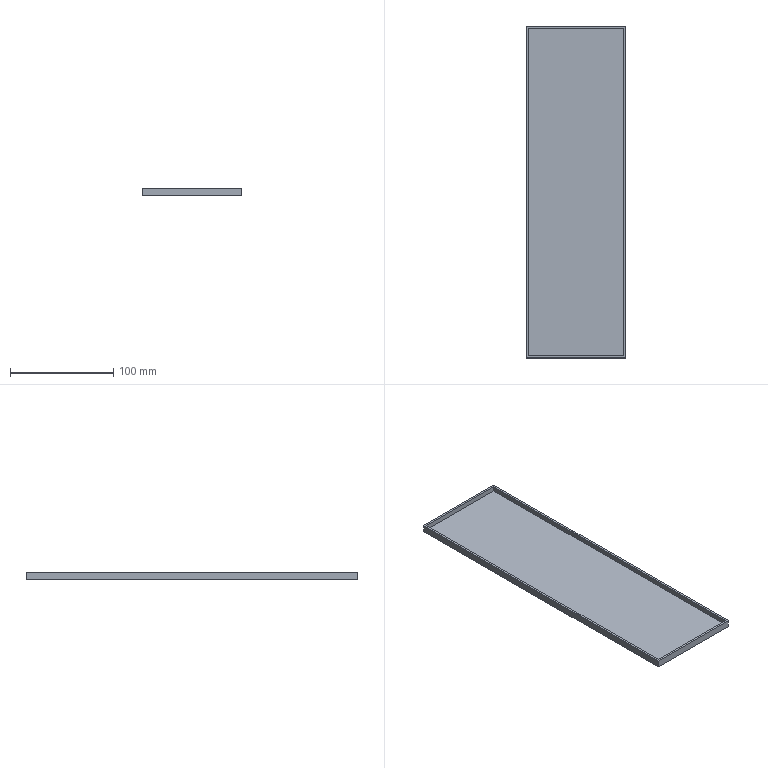Part | NX | features solid 2 | 1 solid | 11 faces | box 96 x 321 x 7 mm | volume 69892 mm3 | plane 11
STEP:
#1=CARTESIAN_POINT('',(-177.,38.,-287.));
#2=VERTEX_POINT('',#1);
#3=CARTESIAN_POINT('',(-177.,-283.,-287.));
#4=VERTEX_POINT('',#3);
#5=CARTESIAN_POINT('',(-177.,-290.,-287.));
#6=DIRECTION('',(0.,-1.,0.));
#7=VECTOR('',#6,1000.);
#8=LINE('',#5,#7);
#9=EDGE_CURVE('',#2,#4,#8,.T.);
#10=ORIENTED_EDGE('',*,*,#9,.F.);
#11=CARTESIAN_POINT('',(-177.,38.,-280.));
#12=VERTEX_POINT('',#11);
#13=CARTESIAN_POINT('',(-177.,38.,-280.));
#14=DIRECTION('',(0.,0.,-1.));
#15=VECTOR('',#14,1000.);
#16=LINE('',#13,#15);
#17=EDGE_CURVE('',#12,#2,#16,.T.);
#18=ORIENTED_EDGE('',*,*,#17,.F.);
#19=CARTESIAN_POINT('',(-177.,-283.,-280.));
#20=VERTEX_POINT('',#19);
#21=CARTESIAN_POINT('',(-177.,-290.,-280.));
#22=DIRECTION('',(0.,-1.,0.));
#23=VECTOR('',#22,1000.);
#24=LINE('',#21,#23);
#25=EDGE_CURVE('',#12,#20,#24,.T.);
#26=ORIENTED_EDGE('',*,*,#25,.T.);
#27=CARTESIAN_POINT('',(-177.,-283.,-280.));
#28=DIRECTION('',(0.,0.,-1.));
#29=VECTOR('',#28,1000.);
#30=LINE('',#27,#29);
#31=EDGE_CURVE('',#20,#4,#30,.T.);
#32=ORIENTED_EDGE('',*,*,#31,.T.);
#33=EDGE_LOOP('',(#10,#18,#26,#32));
#34=FACE_BOUND('',#33,.T.);
#35=CARTESIAN_POINT('',(-177.,35.,-280.));
#36=DIRECTION('',(1.,0.,0.));
#37=DIRECTION('',(0.,0.,-1.));
#38=AXIS2_PLACEMENT_3D('',#35,#36,#37);
#39=PLANE('',#38);
#40=ADVANCED_FACE('',(#34),#39,.T.);
#41=CARTESIAN_POINT('',(-273.,-283.,-287.));
#42=VERTEX_POINT('',#41);
#43=CARTESIAN_POINT('',(-180.,-283.,-287.));
#44=DIRECTION('',(-1.,0.,0.));
#45=VECTOR('',#44,1000.);
#46=LINE('',#43,#45);
#47=EDGE_CURVE('',#4,#42,#46,.T.);
#48=ORIENTED_EDGE('',*,*,#47,.F.);
#49=ORIENTED_EDGE('',*,*,#31,.F.);
#50=CARTESIAN_POINT('',(-273.,-283.,-280.));
#51=VERTEX_POINT('',#50);
#52=CARTESIAN_POINT('',(-180.,-283.,-280.));
#53=DIRECTION('',(-1.,0.,0.));
#54=VECTOR('',#53,1000.);
#55=LINE('',#52,#54);
#56=EDGE_CURVE('',#20,#51,#55,.T.);
#57=ORIENTED_EDGE('',*,*,#56,.T.);
#58=CARTESIAN_POINT('',(-273.,-283.,-280.));
#59=DIRECTION('',(0.,0.,-1.));
#60=VECTOR('',#59,1000.);
#61=LINE('',#58,#60);
#62=EDGE_CURVE('',#51,#42,#61,.T.);
#63=ORIENTED_EDGE('',*,*,#62,.T.);
#64=EDGE_LOOP('',(#48,#49,#57,#63));
#65=FACE_BOUND('',#64,.T.);
#66=CARTESIAN_POINT('',(-690.,-283.,-280.));
#67=DIRECTION('',(0.,-1.,0.));
#68=DIRECTION('',(1.,0.,0.));
#69=AXIS2_PLACEMENT_3D('',#66,#67,#68);
#70=PLANE('',#69);
#71=ADVANCED_FACE('',(#65),#70,.T.);
#72=CARTESIAN_POINT('',(-273.,38.,-287.));
#73=VERTEX_POINT('',#72);
#74=CARTESIAN_POINT('',(-273.,-290.,-287.));
#75=DIRECTION('',(0.,1.,0.));
#76=VECTOR('',#75,1000.);
#77=LINE('',#74,#76);
#78=EDGE_CURVE('',#42,#73,#77,.T.);
#79=ORIENTED_EDGE('',*,*,#78,.F.);
#80=ORIENTED_EDGE('',*,*,#62,.F.);
#81=CARTESIAN_POINT('',(-273.,38.,-280.));
#82=VERTEX_POINT('',#81);
#83=CARTESIAN_POINT('',(-273.,-290.,-280.));
#84=DIRECTION('',(0.,1.,0.));
#85=VECTOR('',#84,1000.);
#86=LINE('',#83,#85);
#87=EDGE_CURVE('',#51,#82,#86,.T.);
#88=ORIENTED_EDGE('',*,*,#87,.T.);
#89=CARTESIAN_POINT('',(-273.,38.,-280.));
#90=DIRECTION('',(0.,0.,-1.));
#91=VECTOR('',#90,1000.);
#92=LINE('',#89,#91);
#93=EDGE_CURVE('',#82,#73,#92,.T.);
#94=ORIENTED_EDGE('',*,*,#93,.T.);
#95=EDGE_LOOP('',(#79,#80,#88,#94));
#96=FACE_BOUND('',#95,.T.);
#97=CARTESIAN_POINT('',(-273.,-290.,-280.));
#98=DIRECTION('',(-1.,0.,0.));
#99=DIRECTION('',(0.,0.,1.));
#100=AXIS2_PLACEMENT_3D('',#97,#98,#99);
#101=PLANE('',#100);
#102=ADVANCED_FACE('',(#96),#101,.T.);
#103=CARTESIAN_POINT('',(-180.,38.,-287.));
#104=DIRECTION('',(1.,0.,0.));
#105=VECTOR('',#104,1000.);
#106=LINE('',#103,#105);
#107=EDGE_CURVE('',#73,#2,#106,.T.);
#108=ORIENTED_EDGE('',*,*,#107,.F.);
#109=ORIENTED_EDGE('',*,*,#93,.F.);
#110=CARTESIAN_POINT('',(-180.,38.,-280.));
#111=DIRECTION('',(1.,0.,0.));
#112=VECTOR('',#111,1000.);
#113=LINE('',#110,#112);
#114=EDGE_CURVE('',#82,#12,#113,.T.);
#115=ORIENTED_EDGE('',*,*,#114,.T.);
#116=ORIENTED_EDGE('',*,*,#17,.T.);
#117=EDGE_LOOP('',(#108,#109,#115,#116));
#118=FACE_BOUND('',#117,.T.);
#119=CARTESIAN_POINT('',(-270.,38.,-280.));
#120=DIRECTION('',(0.,1.,0.));
#121=DIRECTION('',(0.,0.,1.));
#122=AXIS2_PLACEMENT_3D('',#119,#120,#121);
#123=PLANE('',#122);
#124=ADVANCED_FACE('',(#118),#123,.T.);
#125=CARTESIAN_POINT('',(-271.,36.,-280.));
#126=VERTEX_POINT('',#125);
#127=CARTESIAN_POINT('',(-179.,36.,-280.));
#128=VERTEX_POINT('',#127);
#129=CARTESIAN_POINT('',(-180.,36.,-280.));
#130=DIRECTION('',(1.,0.,0.));
#131=VECTOR('',#130,1000.);
#132=LINE('',#129,#131);
#133=EDGE_CURVE('',#126,#128,#132,.T.);
#134=ORIENTED_EDGE('',*,*,#133,.T.);
#135=CARTESIAN_POINT('',(-179.,-281.,-280.));
#136=VERTEX_POINT('',#135);
#137=CARTESIAN_POINT('',(-179.,-290.,-280.));
#138=DIRECTION('',(0.,-1.,0.));
#139=VECTOR('',#138,1000.);
#140=LINE('',#137,#139);
#141=EDGE_CURVE('',#128,#136,#140,.T.);
#142=ORIENTED_EDGE('',*,*,#141,.T.);
#143=CARTESIAN_POINT('',(-271.,-281.,-280.));
#144=VERTEX_POINT('',#143);
#145=CARTESIAN_POINT('',(-180.,-281.,-280.));
#146=DIRECTION('',(-1.,0.,0.));
#147=VECTOR('',#146,1000.);
#148=LINE('',#145,#147);
#149=EDGE_CURVE('',#136,#144,#148,.T.);
#150=ORIENTED_EDGE('',*,*,#149,.T.);
#151=CARTESIAN_POINT('',(-271.,-290.,-280.));
#152=DIRECTION('',(0.,1.,0.));
#153=VECTOR('',#152,1000.);
#154=LINE('',#151,#153);
#155=EDGE_CURVE('',#144,#126,#154,.T.);
#156=ORIENTED_EDGE('',*,*,#155,.T.);
#157=EDGE_LOOP('',(#134,#142,#150,#156));
#158=FACE_BOUND('',#157,.T.);
#159=ORIENTED_EDGE('',*,*,#25,.F.);
#160=ORIENTED_EDGE('',*,*,#114,.F.);
#161=ORIENTED_EDGE('',*,*,#87,.F.);
#162=ORIENTED_EDGE('',*,*,#56,.F.);
#163=EDGE_LOOP('',(#159,#160,#161,#162));
#164=FACE_BOUND('',#163,.T.);
#165=CARTESIAN_POINT('',(-180.,-290.,-280.));
#166=DIRECTION('',(0.,0.,-1.));
#167=DIRECTION('',(-1.,0.,0.));
#168=AXIS2_PLACEMENT_3D('',#165,#166,#167);
#169=PLANE('',#168);
#170=ADVANCED_FACE('',(#158,#164),#169,.F.);
#171=ORIENTED_EDGE('',*,*,#9,.T.);
#172=ORIENTED_EDGE('',*,*,#47,.T.);
#173=ORIENTED_EDGE('',*,*,#78,.T.);
#174=ORIENTED_EDGE('',*,*,#107,.T.);
#175=EDGE_LOOP('',(#171,#172,#173,#174));
#176=FACE_BOUND('',#175,.T.);
#177=CARTESIAN_POINT('',(-180.,-290.,-287.));
#178=DIRECTION('',(0.,0.,-1.));
#179=DIRECTION('',(-1.,0.,0.));
#180=AXIS2_PLACEMENT_3D('',#177,#178,#179);
#181=PLANE('',#180);
#182=ADVANCED_FACE('',(#176),#181,.T.);
#183=CARTESIAN_POINT('',(-179.,36.,-285.));
#184=VERTEX_POINT('',#183);
#185=CARTESIAN_POINT('',(-179.,-281.,-285.));
#186=VERTEX_POINT('',#185);
#187=CARTESIAN_POINT('',(-179.,-290.,-285.));
#188=DIRECTION('',(0.,-1.,0.));
#189=VECTOR('',#188,1000.);
#190=LINE('',#187,#189);
#191=EDGE_CURVE('',#184,#186,#190,.T.);
#192=ORIENTED_EDGE('',*,*,#191,.T.);
#193=CARTESIAN_POINT('',(-179.,-281.,-280.));
#194=DIRECTION('',(0.,0.,-1.));
#195=VECTOR('',#194,1000.);
#196=LINE('',#193,#195);
#197=EDGE_CURVE('',#136,#186,#196,.T.);
#198=ORIENTED_EDGE('',*,*,#197,.F.);
#199=ORIENTED_EDGE('',*,*,#141,.F.);
#200=CARTESIAN_POINT('',(-179.,36.,-280.));
#201=DIRECTION('',(0.,0.,-1.));
#202=VECTOR('',#201,1000.);
#203=LINE('',#200,#202);
#204=EDGE_CURVE('',#128,#184,#203,.T.);
#205=ORIENTED_EDGE('',*,*,#204,.T.);
#206=EDGE_LOOP('',(#192,#198,#199,#205));
#207=FACE_BOUND('',#206,.T.);
#208=CARTESIAN_POINT('',(-179.,35.,-280.));
#209=DIRECTION('',(1.,0.,0.));
#210=DIRECTION('',(0.,0.,-1.));
#211=AXIS2_PLACEMENT_3D('',#208,#209,#210);
#212=PLANE('',#211);
#213=ADVANCED_FACE('',(#207),#212,.F.);
#214=CARTESIAN_POINT('',(-271.,-281.,-285.));
#215=VERTEX_POINT('',#214);
#216=CARTESIAN_POINT('',(-180.,-281.,-285.));
#217=DIRECTION('',(-1.,0.,0.));
#218=VECTOR('',#217,1000.);
#219=LINE('',#216,#218);
#220=EDGE_CURVE('',#186,#215,#219,.T.);
#221=ORIENTED_EDGE('',*,*,#220,.T.);
#222=CARTESIAN_POINT('',(-271.,-281.,-280.));
#223=DIRECTION('',(0.,0.,-1.));
#224=VECTOR('',#223,1000.);
#225=LINE('',#222,#224);
#226=EDGE_CURVE('',#144,#215,#225,.T.);
#227=ORIENTED_EDGE('',*,*,#226,.F.);
#228=ORIENTED_EDGE('',*,*,#149,.F.);
#229=ORIENTED_EDGE('',*,*,#197,.T.);
#230=EDGE_LOOP('',(#221,#227,#228,#229));
#231=FACE_BOUND('',#230,.T.);
#232=CARTESIAN_POINT('',(-690.,-281.,-280.));
#233=DIRECTION('',(0.,-1.,0.));
#234=DIRECTION('',(1.,0.,0.));
#235=AXIS2_PLACEMENT_3D('',#232,#233,#234);
#236=PLANE('',#235);
#237=ADVANCED_FACE('',(#231),#236,.F.);
#238=CARTESIAN_POINT('',(-271.,36.,-285.));
#239=VERTEX_POINT('',#238);
#240=CARTESIAN_POINT('',(-271.,-290.,-285.));
#241=DIRECTION('',(0.,1.,0.));
#242=VECTOR('',#241,1000.);
#243=LINE('',#240,#242);
#244=EDGE_CURVE('',#215,#239,#243,.T.);
#245=ORIENTED_EDGE('',*,*,#244,.T.);
#246=CARTESIAN_POINT('',(-271.,36.,-280.));
#247=DIRECTION('',(0.,0.,-1.));
#248=VECTOR('',#247,1000.);
#249=LINE('',#246,#248);
#250=EDGE_CURVE('',#126,#239,#249,.T.);
#251=ORIENTED_EDGE('',*,*,#250,.F.);
#252=ORIENTED_EDGE('',*,*,#155,.F.);
#253=ORIENTED_EDGE('',*,*,#226,.T.);
#254=EDGE_LOOP('',(#245,#251,#252,#253));
#255=FACE_BOUND('',#254,.T.);
#256=CARTESIAN_POINT('',(-271.,-290.,-280.));
#257=DIRECTION('',(-1.,0.,0.));
#258=DIRECTION('',(0.,0.,1.));
#259=AXIS2_PLACEMENT_3D('',#256,#257,#258);
#260=PLANE('',#259);
#261=ADVANCED_FACE('',(#255),#260,.F.);
#262=CARTESIAN_POINT('',(-180.,36.,-285.));
#263=DIRECTION('',(1.,0.,0.));
#264=VECTOR('',#263,1000.);
#265=LINE('',#262,#264);
#266=EDGE_CURVE('',#239,#184,#265,.T.);
#267=ORIENTED_EDGE('',*,*,#266,.T.);
#268=ORIENTED_EDGE('',*,*,#204,.F.);
#269=ORIENTED_EDGE('',*,*,#133,.F.);
#270=ORIENTED_EDGE('',*,*,#250,.T.);
#271=EDGE_LOOP('',(#267,#268,#269,#270));
#272=FACE_BOUND('',#271,.T.);
#273=CARTESIAN_POINT('',(-270.,36.,-280.));
#274=DIRECTION('',(0.,1.,0.));
#275=DIRECTION('',(0.,0.,1.));
#276=AXIS2_PLACEMENT_3D('',#273,#274,#275);
#277=PLANE('',#276);
#278=ADVANCED_FACE('',(#272),#277,.F.);
#279=ORIENTED_EDGE('',*,*,#191,.F.);
#280=ORIENTED_EDGE('',*,*,#266,.F.);
#281=ORIENTED_EDGE('',*,*,#244,.F.);
#282=ORIENTED_EDGE('',*,*,#220,.F.);
#283=EDGE_LOOP('',(#279,#280,#281,#282));
#284=FACE_BOUND('',#283,.T.);
#285=CARTESIAN_POINT('',(-180.,-290.,-285.));
#286=DIRECTION('',(0.,0.,-1.));
#287=DIRECTION('',(-1.,0.,0.));
#288=AXIS2_PLACEMENT_3D('',#285,#286,#287);
#289=PLANE('',#288);
#290=ADVANCED_FACE('',(#284),#289,.F.);
#291=CLOSED_SHELL('',(#40,#71,#102,#124,#170,#182,#213,#237,#261,#278,#290));
#292=MANIFOLD_SOLID_BREP('',#291);
#293=(LENGTH_UNIT()NAMED_UNIT(*)SI_UNIT(.MILLI.,.METRE.));
#294=UNCERTAINTY_MEASURE_WITH_UNIT(LENGTH_MEASURE(0.00001),#293,'','');
#295=(NAMED_UNIT(*)PLANE_ANGLE_UNIT()SI_UNIT($,.RADIAN.));
#296=(NAMED_UNIT(*)SI_UNIT($,.STERADIAN.)SOLID_ANGLE_UNIT());
#297=(GEOMETRIC_REPRESENTATION_CONTEXT(3)GLOBAL_UNCERTAINTY_ASSIGNED_CONTEXT((#294))GLOBAL_UNIT_ASSIGNED_CONTEXT((#293,#295,#296))REPRESENTATION_CONTEXT('',''));
#298=ADVANCED_BREP_SHAPE_REPRESENTATION('',(#292),#297);